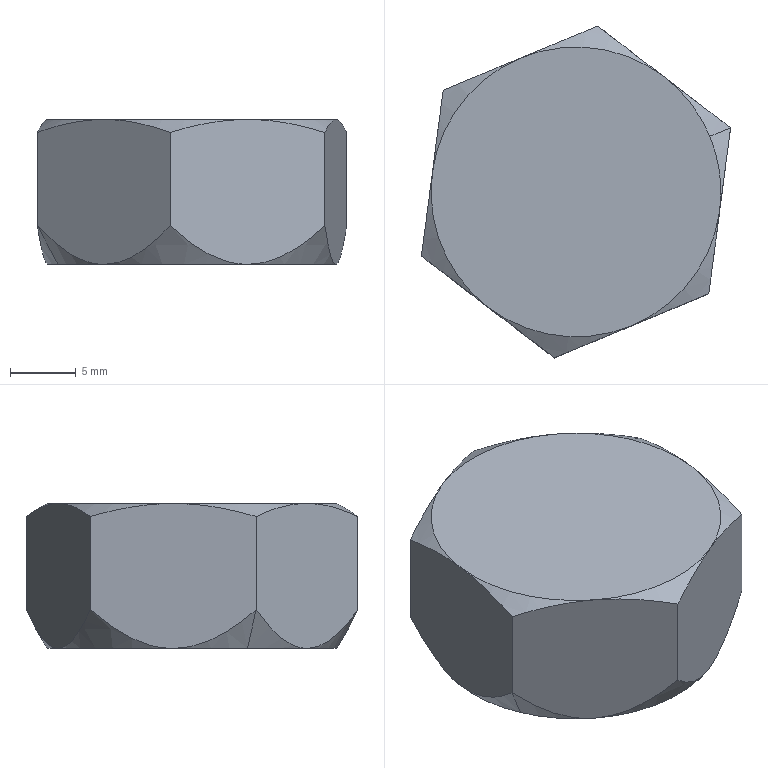Part | SolidWorks | features BaseBody 1 | 1 solid | 30 faces | box 23.463 x 25.189 x 11 mm | volume 2187 mm3 | cone 16 | plane 10 | cylinder 4 | commonest cylinder face diameters 18 x2 19 x2
STEP:
#1=CARTESIAN_POINT('',(-48.302,46.11,95.75));
#2=VERTEX_POINT('',#1);
#3=CARTESIAN_POINT('',(-51.768,50.624,95.75));
#4=VERTEX_POINT('',#3);
#5=CARTESIAN_POINT('',(-58.463,41.896,95.75));
#6=DIRECTION('',(0.,0.,1.));
#7=DIRECTION('',(0.9237,0.383,0.));
#8=AXIS2_PLACEMENT_3D('',#5,#6,#7);
#9=CIRCLE('',#8,11.);
#10=EDGE_CURVE('',#2,#4,#9,.T.);
#11=ORIENTED_EDGE('',*,*,#10,.F.);
#12=CARTESIAN_POINT('',(-46.732,46.761,94.769));
#13=VERTEX_POINT('',#12);
#14=CARTESIAN_POINT('',(-48.302,46.11,95.75));
#15=DIRECTION('',(0.8,0.3317,-0.5));
#16=VECTOR('',#15,1000.);
#17=LINE('',#14,#16);
#18=EDGE_CURVE('',#2,#13,#17,.T.);
#19=ORIENTED_EDGE('',*,*,#18,.T.);
#20=CARTESIAN_POINT('',(-51.768,50.624,95.75));
#21=CARTESIAN_POINT('',(-50.908,49.965,95.75));
#22=CARTESIAN_POINT('',(-50.06,49.314,95.656));
#23=CARTESIAN_POINT('',(-48.383,48.028,95.314));
#24=CARTESIAN_POINT('',(-47.554,47.392,95.068));
#25=CARTESIAN_POINT('',(-46.732,46.761,94.769));
#26=B_SPLINE_CURVE_WITH_KNOTS('',3,(#20,#21,#22,#23,#24,#25),.UNSPECIFIED.,.F.,.F.,(4,2,4),(0.,0.003211,0.006423),.UNSPECIFIED.);
#27=EDGE_CURVE('',#4,#13,#26,.T.);
#28=ORIENTED_EDGE('',*,*,#27,.F.);
#29=EDGE_LOOP('',(#11,#19,#28));
#30=FACE_OUTER_BOUND('',#29,.T.);
#31=CARTESIAN_POINT('',(-58.463,41.896,95.75));
#32=DIRECTION('',(0.,0.,-1.));
#33=DIRECTION('',(0.9237,0.383,0.));
#34=AXIS2_PLACEMENT_3D('',#31,#32,#33);
#35=CONICAL_SURFACE('',#34,11.,1.047);
#36=ADVANCED_FACE('',(#30),#35,.T.);
#37=CARTESIAN_POINT('',(-68.624,37.683,84.75));
#38=VERTEX_POINT('',#37);
#39=CARTESIAN_POINT('',(-69.37,43.325,84.75));
#40=VERTEX_POINT('',#39);
#41=CARTESIAN_POINT('',(-58.463,41.896,84.75));
#42=DIRECTION('',(0.,0.,-1.));
#43=DIRECTION('',(-0.9237,-0.383,0.));
#44=AXIS2_PLACEMENT_3D('',#41,#42,#43);
#45=CIRCLE('',#44,11.);
#46=EDGE_CURVE('',#38,#40,#45,.T.);
#47=ORIENTED_EDGE('',*,*,#46,.F.);
#48=CARTESIAN_POINT('',(-70.194,37.031,87.694));
#49=VERTEX_POINT('',#48);
#50=CARTESIAN_POINT('',(-68.624,37.683,84.75));
#51=DIRECTION('',(-0.4619,-0.1915,0.866));
#52=VECTOR('',#51,1000.);
#53=LINE('',#50,#52);
#54=EDGE_CURVE('',#38,#49,#53,.T.);
#55=ORIENTED_EDGE('',*,*,#54,.T.);
#56=CARTESIAN_POINT('',(-69.37,43.325,84.75));
#57=CARTESIAN_POINT('',(-69.448,42.726,84.75));
#58=CARTESIAN_POINT('',(-69.524,42.145,84.836));
#59=CARTESIAN_POINT('',(-69.636,41.292,85.072));
#60=CARTESIAN_POINT('',(-69.673,41.011,85.168));
#61=CARTESIAN_POINT('',(-69.745,40.458,85.392));
#62=CARTESIAN_POINT('',(-69.78,40.19,85.517));
#63=CARTESIAN_POINT('',(-69.883,39.404,85.925));
#64=CARTESIAN_POINT('',(-69.949,38.906,86.24));
#65=CARTESIAN_POINT('',(-70.075,37.944,86.929));
#66=CARTESIAN_POINT('',(-70.135,37.48,87.303));
#67=CARTESIAN_POINT('',(-70.194,37.031,87.694));
#68=B_SPLINE_CURVE_WITH_KNOTS('',3,(#56,#57,#58,#59,#60,#61,#62,#63,#64,#65,#66,#67),.UNSPECIFIED.,.F.,.F.,(4,2,2,2,2,4),(0.,0.001777,0.002666,0.003555,0.005332,0.00711),.UNSPECIFIED.);
#69=EDGE_CURVE('',#40,#49,#68,.T.);
#70=ORIENTED_EDGE('',*,*,#69,.F.);
#71=EDGE_LOOP('',(#47,#55,#70));
#72=FACE_OUTER_BOUND('',#71,.T.);
#73=CARTESIAN_POINT('',(-58.463,41.896,84.75));
#74=DIRECTION('',(0.,0.,1.));
#75=DIRECTION('',(-0.9237,-0.383,0.));
#76=AXIS2_PLACEMENT_3D('',#73,#74,#75);
#77=CONICAL_SURFACE('',#76,11.,0.5236);
#78=ADVANCED_FACE('',(#72),#77,.T.);
#79=CARTESIAN_POINT('',(-66.776,38.449,91.75));
#80=VERTEX_POINT('',#79);
#81=CARTESIAN_POINT('',(-50.149,45.344,91.75));
#82=VERTEX_POINT('',#81);
#83=CARTESIAN_POINT('',(-58.463,41.896,91.75));
#84=DIRECTION('',(0.,0.,1.));
#85=DIRECTION('',(0.9237,0.383,0.));
#86=AXIS2_PLACEMENT_3D('',#83,#84,#85);
#87=CIRCLE('',#86,9.);
#88=EDGE_CURVE('',#80,#82,#87,.T.);
#89=ORIENTED_EDGE('',*,*,#88,.T.);
#90=CARTESIAN_POINT('',(-50.149,45.344,85.75));
#91=VERTEX_POINT('',#90);
#92=CARTESIAN_POINT('',(-50.149,45.344,93.75));
#93=DIRECTION('',(0.,0.,-1.));
#94=VECTOR('',#93,1000.);
#95=LINE('',#92,#94);
#96=EDGE_CURVE('',#82,#91,#95,.T.);
#97=ORIENTED_EDGE('',*,*,#96,.T.);
#98=CARTESIAN_POINT('',(-66.776,38.449,85.75));
#99=VERTEX_POINT('',#98);
#100=CARTESIAN_POINT('',(-58.463,41.896,85.75));
#101=DIRECTION('',(0.,0.,-1.));
#102=DIRECTION('',(0.9237,0.383,0.));
#103=AXIS2_PLACEMENT_3D('',#100,#101,#102);
#104=CIRCLE('',#103,9.);
#105=EDGE_CURVE('',#91,#99,#104,.T.);
#106=ORIENTED_EDGE('',*,*,#105,.T.);
#107=CARTESIAN_POINT('',(-66.776,38.449,93.75));
#108=DIRECTION('',(0.,0.,-1.));
#109=VECTOR('',#108,1000.);
#110=LINE('',#107,#109);
#111=EDGE_CURVE('',#80,#99,#110,.T.);
#112=ORIENTED_EDGE('',*,*,#111,.F.);
#113=EDGE_LOOP('',(#89,#97,#106,#112));
#114=FACE_OUTER_BOUND('',#113,.T.);
#115=CARTESIAN_POINT('',(-58.463,41.896,93.75));
#116=DIRECTION('',(0.,0.,-1.));
#117=DIRECTION('',(-0.9237,-0.383,0.));
#118=AXIS2_PLACEMENT_3D('',#115,#116,#117);
#119=CYLINDRICAL_SURFACE('',#118,9.);
#120=ADVANCED_FACE('',(#114),#119,.F.);
#121=CARTESIAN_POINT('',(-67.238,38.257,91.75));
#122=VERTEX_POINT('',#121);
#123=CARTESIAN_POINT('',(-49.687,45.535,91.75));
#124=VERTEX_POINT('',#123);
#125=CARTESIAN_POINT('',(-58.463,41.896,91.75));
#126=DIRECTION('',(0.,0.,1.));
#127=DIRECTION('',(0.9237,0.383,0.));
#128=AXIS2_PLACEMENT_3D('',#125,#126,#127);
#129=CIRCLE('',#128,9.5);
#130=EDGE_CURVE('',#122,#124,#129,.T.);
#131=ORIENTED_EDGE('',*,*,#130,.F.);
#132=CARTESIAN_POINT('',(-67.238,38.257,93.75));
#133=VERTEX_POINT('',#132);
#134=CARTESIAN_POINT('',(-67.238,38.257,91.75));
#135=DIRECTION('',(0.,0.,1.));
#136=VECTOR('',#135,1000.);
#137=LINE('',#134,#136);
#138=EDGE_CURVE('',#122,#133,#137,.T.);
#139=ORIENTED_EDGE('',*,*,#138,.T.);
#140=CARTESIAN_POINT('',(-49.687,45.535,93.75));
#141=VERTEX_POINT('',#140);
#142=CARTESIAN_POINT('',(-58.463,41.896,93.75));
#143=DIRECTION('',(0.,0.,1.));
#144=DIRECTION('',(0.9237,0.383,0.));
#145=AXIS2_PLACEMENT_3D('',#142,#143,#144);
#146=CIRCLE('',#145,9.5);
#147=EDGE_CURVE('',#133,#141,#146,.T.);
#148=ORIENTED_EDGE('',*,*,#147,.T.);
#149=CARTESIAN_POINT('',(-49.687,45.535,91.75));
#150=DIRECTION('',(0.,0.,1.));
#151=VECTOR('',#150,1000.);
#152=LINE('',#149,#151);
#153=EDGE_CURVE('',#124,#141,#152,.T.);
#154=ORIENTED_EDGE('',*,*,#153,.F.);
#155=EDGE_LOOP('',(#131,#139,#148,#154));
#156=FACE_OUTER_BOUND('',#155,.T.);
#157=CARTESIAN_POINT('',(-58.463,41.896,91.75));
#158=DIRECTION('',(0.,0.,1.));
#159=DIRECTION('',(0.9237,0.383,0.));
#160=AXIS2_PLACEMENT_3D('',#157,#158,#159);
#161=CYLINDRICAL_SURFACE('',#160,9.5);
#162=ADVANCED_FACE('',(#156),#161,.F.);
#163=ORIENTED_EDGE('',*,*,#105,.F.);
#164=CARTESIAN_POINT('',(-49.226,45.727,84.75));
#165=VERTEX_POINT('',#164);
#166=CARTESIAN_POINT('',(-50.149,45.344,85.75));
#167=DIRECTION('',(0.6532,0.2709,-0.7071));
#168=VECTOR('',#167,1000.);
#169=LINE('',#166,#168);
#170=EDGE_CURVE('',#91,#165,#169,.T.);
#171=ORIENTED_EDGE('',*,*,#170,.T.);
#172=CARTESIAN_POINT('',(-67.7,38.066,84.75));
#173=VERTEX_POINT('',#172);
#174=CARTESIAN_POINT('',(-58.463,41.896,84.75));
#175=DIRECTION('',(0.,0.,1.));
#176=DIRECTION('',(0.9237,0.383,0.));
#177=AXIS2_PLACEMENT_3D('',#174,#175,#176);
#178=CIRCLE('',#177,10.);
#179=EDGE_CURVE('',#173,#165,#178,.T.);
#180=ORIENTED_EDGE('',*,*,#179,.F.);
#181=CARTESIAN_POINT('',(-66.776,38.449,85.75));
#182=DIRECTION('',(-0.6532,-0.2709,-0.7071));
#183=VECTOR('',#182,1000.);
#184=LINE('',#181,#183);
#185=EDGE_CURVE('',#99,#173,#184,.T.);
#186=ORIENTED_EDGE('',*,*,#185,.F.);
#187=EDGE_LOOP('',(#163,#171,#180,#186));
#188=FACE_OUTER_BOUND('',#187,.T.);
#189=CARTESIAN_POINT('',(-58.463,41.896,85.75));
#190=DIRECTION('',(0.,0.,-1.));
#191=DIRECTION('',(-0.9237,-0.383,0.));
#192=AXIS2_PLACEMENT_3D('',#189,#190,#191);
#193=CONICAL_SURFACE('',#192,9.,0.7854);
#194=ADVANCED_FACE('',(#188),#193,.F.);
#195=ORIENTED_EDGE('',*,*,#170,.F.);
#196=CARTESIAN_POINT('',(-58.463,41.896,85.75));
#197=DIRECTION('',(0.,0.,-1.));
#198=DIRECTION('',(0.9237,0.383,0.));
#199=AXIS2_PLACEMENT_3D('',#196,#197,#198);
#200=CIRCLE('',#199,9.);
#201=EDGE_CURVE('',#99,#91,#200,.T.);
#202=ORIENTED_EDGE('',*,*,#201,.F.);
#203=ORIENTED_EDGE('',*,*,#185,.T.);
#204=CARTESIAN_POINT('',(-58.463,41.896,84.75));
#205=DIRECTION('',(0.,0.,1.));
#206=DIRECTION('',(0.9237,0.383,0.));
#207=AXIS2_PLACEMENT_3D('',#204,#205,#206);
#208=CIRCLE('',#207,10.);
#209=EDGE_CURVE('',#165,#173,#208,.T.);
#210=ORIENTED_EDGE('',*,*,#209,.F.);
#211=EDGE_LOOP('',(#195,#202,#203,#210));
#212=FACE_OUTER_BOUND('',#211,.T.);
#213=CARTESIAN_POINT('',(-58.463,41.896,85.75));
#214=DIRECTION('',(0.,0.,-1.));
#215=DIRECTION('',(-0.9237,-0.383,0.));
#216=AXIS2_PLACEMENT_3D('',#213,#214,#215);
#217=CONICAL_SURFACE('',#216,9.,0.7854);
#218=ADVANCED_FACE('',(#212),#217,.F.);
#219=CARTESIAN_POINT('',(-58.463,41.896,93.75));
#220=DIRECTION('',(0.,0.,1.));
#221=DIRECTION('',(0.9237,0.383,0.));
#222=AXIS2_PLACEMENT_3D('',#219,#220,#221);
#223=CIRCLE('',#222,9.5);
#224=EDGE_CURVE('',#141,#133,#223,.T.);
#225=ORIENTED_EDGE('',*,*,#224,.F.);
#226=ORIENTED_EDGE('',*,*,#147,.F.);
#227=EDGE_LOOP('',(#225,#226));
#228=FACE_OUTER_BOUND('',#227,.T.);
#229=CARTESIAN_POINT('',(-58.463,41.896,93.75));
#230=DIRECTION('',(0.,0.,1.));
#231=DIRECTION('',(1.,0.,0.));
#232=AXIS2_PLACEMENT_3D('',#229,#230,#231);
#233=PLANE('',#232);
#234=ADVANCED_FACE('',(#228),#233,.F.);
#235=CARTESIAN_POINT('',(-58.463,41.896,91.75));
#236=DIRECTION('',(0.,0.,1.));
#237=DIRECTION('',(0.9237,0.383,0.));
#238=AXIS2_PLACEMENT_3D('',#235,#236,#237);
#239=CIRCLE('',#238,9.5);
#240=EDGE_CURVE('',#124,#122,#239,.T.);
#241=ORIENTED_EDGE('',*,*,#240,.T.);
#242=ORIENTED_EDGE('',*,*,#130,.T.);
#243=EDGE_LOOP('',(#241,#242));
#244=FACE_OUTER_BOUND('',#243,.T.);
#245=ORIENTED_EDGE('',*,*,#88,.F.);
#246=CARTESIAN_POINT('',(-58.463,41.896,91.75));
#247=DIRECTION('',(0.,0.,1.));
#248=DIRECTION('',(0.9237,0.383,0.));
#249=AXIS2_PLACEMENT_3D('',#246,#247,#248);
#250=CIRCLE('',#249,9.);
#251=EDGE_CURVE('',#82,#80,#250,.T.);
#252=ORIENTED_EDGE('',*,*,#251,.F.);
#253=EDGE_LOOP('',(#245,#252));
#254=FACE_BOUND('',#253,.T.);
#255=CARTESIAN_POINT('',(-58.463,41.896,91.75));
#256=DIRECTION('',(0.,0.,1.));
#257=DIRECTION('',(1.,0.,0.));
#258=AXIS2_PLACEMENT_3D('',#255,#256,#257);
#259=PLANE('',#258);
#260=ADVANCED_FACE('',(#244,#254),#259,.T.);
#261=ORIENTED_EDGE('',*,*,#138,.F.);
#262=ORIENTED_EDGE('',*,*,#240,.F.);
#263=ORIENTED_EDGE('',*,*,#153,.T.);
#264=ORIENTED_EDGE('',*,*,#224,.T.);
#265=EDGE_LOOP('',(#261,#262,#263,#264));
#266=FACE_OUTER_BOUND('',#265,.T.);
#267=CARTESIAN_POINT('',(-58.463,41.896,91.75));
#268=DIRECTION('',(0.,0.,1.));
#269=DIRECTION('',(0.9237,0.383,0.));
#270=AXIS2_PLACEMENT_3D('',#267,#268,#269);
#271=CYLINDRICAL_SURFACE('',#270,9.5);
#272=ADVANCED_FACE('',(#266),#271,.F.);
#273=ORIENTED_EDGE('',*,*,#96,.F.);
#274=ORIENTED_EDGE('',*,*,#251,.T.);
#275=ORIENTED_EDGE('',*,*,#111,.T.);
#276=ORIENTED_EDGE('',*,*,#201,.T.);
#277=EDGE_LOOP('',(#273,#274,#275,#276));
#278=FACE_OUTER_BOUND('',#277,.T.);
#279=CARTESIAN_POINT('',(-58.463,41.896,93.75));
#280=DIRECTION('',(0.,0.,-1.));
#281=DIRECTION('',(-0.9237,-0.383,0.));
#282=AXIS2_PLACEMENT_3D('',#279,#280,#281);
#283=CYLINDRICAL_SURFACE('',#282,9.);
#284=ADVANCED_FACE('',(#278),#283,.F.);
#285=CARTESIAN_POINT('',(-56.808,54.491,87.699));
#286=VERTEX_POINT('',#285);
#287=CARTESIAN_POINT('',(-62.676,52.057,84.75));
#288=VERTEX_POINT('',#287);
#289=CARTESIAN_POINT('',(-56.808,54.491,87.699));
#290=CARTESIAN_POINT('',(-57.226,54.318,87.308));
#291=CARTESIAN_POINT('',(-57.655,54.14,86.936));
#292=CARTESIAN_POINT('',(-58.548,53.769,86.249));
#293=CARTESIAN_POINT('',(-59.011,53.577,85.933));
#294=CARTESIAN_POINT('',(-59.744,53.273,85.523));
#295=CARTESIAN_POINT('',(-59.996,53.169,85.396));
#296=CARTESIAN_POINT('',(-60.511,52.955,85.172));
#297=CARTESIAN_POINT('',(-60.772,52.847,85.076));
#298=CARTESIAN_POINT('',(-61.302,52.627,84.917));
#299=CARTESIAN_POINT('',(-61.571,52.516,84.856));
#300=CARTESIAN_POINT('',(-62.118,52.289,84.772));
#301=CARTESIAN_POINT('',(-62.397,52.173,84.75));
#302=CARTESIAN_POINT('',(-62.676,52.057,84.75));
#303=B_SPLINE_CURVE_WITH_KNOTS('',3,(#289,#290,#291,#292,#293,#294,#295,#296,#297,#298,#299,#300,#301,#302),.UNSPECIFIED.,.F.,.F.,(4,2,2,2,2,2,4),(0.,0.001777,0.003555,0.004444,0.005332,0.006221,0.00711),.UNSPECIFIED.);
#304=EDGE_CURVE('',#286,#288,#303,.T.);
#305=ORIENTED_EDGE('',*,*,#304,.F.);
#306=CARTESIAN_POINT('',(-51.768,50.624,84.75));
#307=VERTEX_POINT('',#306);
#308=CARTESIAN_POINT('',(-51.768,50.624,84.75));
#309=CARTESIAN_POINT('',(-52.247,50.992,84.75));
#310=CARTESIAN_POINT('',(-52.714,51.35,84.836));
#311=CARTESIAN_POINT('',(-53.396,51.873,85.072));
#312=CARTESIAN_POINT('',(-53.622,52.046,85.169));
#313=CARTESIAN_POINT('',(-54.064,52.386,85.393));
#314=CARTESIAN_POINT('',(-54.279,52.551,85.518));
#315=CARTESIAN_POINT('',(-54.909,53.033,85.927));
#316=CARTESIAN_POINT('',(-55.307,53.339,86.243));
#317=CARTESIAN_POINT('',(-56.078,53.93,86.932));
#318=CARTESIAN_POINT('',(-56.449,54.215,87.307));
#319=CARTESIAN_POINT('',(-56.808,54.491,87.699));
#320=B_SPLINE_CURVE_WITH_KNOTS('',3,(#308,#309,#310,#311,#312,#313,#314,#315,#316,#317,#318,#319),.UNSPECIFIED.,.F.,.F.,(4,2,2,2,2,4),(0.,0.001779,0.002669,0.003558,0.005337,0.007116),.UNSPECIFIED.);
#321=EDGE_CURVE('',#307,#286,#320,.T.);
#322=ORIENTED_EDGE('',*,*,#321,.F.);
#323=CARTESIAN_POINT('',(-58.463,41.896,84.75));
#324=DIRECTION('',(0.,0.,-1.));
#325=DIRECTION('',(-0.9237,-0.383,0.));
#326=AXIS2_PLACEMENT_3D('',#323,#324,#325);
#327=CIRCLE('',#326,11.);
#328=EDGE_CURVE('',#288,#307,#327,.T.);
#329=ORIENTED_EDGE('',*,*,#328,.F.);
#330=EDGE_LOOP('',(#305,#322,#329));
#331=FACE_OUTER_BOUND('',#330,.T.);
#332=CARTESIAN_POINT('',(-58.463,41.896,84.75));
#333=DIRECTION('',(0.,0.,1.));
#334=DIRECTION('',(-0.9237,-0.383,0.));
#335=AXIS2_PLACEMENT_3D('',#332,#333,#334);
#336=CONICAL_SURFACE('',#335,11.,0.5236);
#337=ADVANCED_FACE('',(#331),#336,.T.);
#338=CARTESIAN_POINT('',(-68.544,49.624,87.699));
#339=VERTEX_POINT('',#338);
#340=CARTESIAN_POINT('',(-62.676,52.057,84.75));
#341=CARTESIAN_POINT('',(-63.235,51.826,84.75));
#342=CARTESIAN_POINT('',(-63.777,51.601,84.836));
#343=CARTESIAN_POINT('',(-64.572,51.271,85.072));
#344=CARTESIAN_POINT('',(-64.834,51.162,85.169));
#345=CARTESIAN_POINT('',(-65.35,50.949,85.393));
#346=CARTESIAN_POINT('',(-65.6,50.845,85.518));
#347=CARTESIAN_POINT('',(-66.333,50.541,85.927));
#348=CARTESIAN_POINT('',(-66.797,50.348,86.243));
#349=CARTESIAN_POINT('',(-67.694,49.977,86.932));
#350=CARTESIAN_POINT('',(-68.126,49.797,87.307));
#351=CARTESIAN_POINT('',(-68.544,49.624,87.699));
#352=B_SPLINE_CURVE_WITH_KNOTS('',3,(#340,#341,#342,#343,#344,#345,#346,#347,#348,#349,#350,#351),.UNSPECIFIED.,.F.,.F.,(4,2,2,2,2,4),(0.,0.001779,0.002669,0.003558,0.005337,0.007116),.UNSPECIFIED.);
#353=EDGE_CURVE('',#288,#339,#352,.T.);
#354=ORIENTED_EDGE('',*,*,#353,.F.);
#355=CARTESIAN_POINT('',(-58.463,41.896,84.75));
#356=DIRECTION('',(0.,0.,-1.));
#357=DIRECTION('',(-0.9237,-0.383,0.));
#358=AXIS2_PLACEMENT_3D('',#355,#356,#357);
#359=CIRCLE('',#358,11.);
#360=EDGE_CURVE('',#40,#288,#359,.T.);
#361=ORIENTED_EDGE('',*,*,#360,.F.);
#362=CARTESIAN_POINT('',(-68.544,49.624,87.699));
#363=CARTESIAN_POINT('',(-68.603,49.176,87.308));
#364=CARTESIAN_POINT('',(-68.663,48.715,86.936));
#365=CARTESIAN_POINT('',(-68.789,47.757,86.249));
#366=CARTESIAN_POINT('',(-68.854,47.26,85.933));
#367=CARTESIAN_POINT('',(-68.957,46.473,85.523));
#368=CARTESIAN_POINT('',(-68.993,46.202,85.396));
#369=CARTESIAN_POINT('',(-69.065,45.649,85.172));
#370=CARTESIAN_POINT('',(-69.102,45.369,85.076));
#371=CARTESIAN_POINT('',(-69.176,44.801,84.917));
#372=CARTESIAN_POINT('',(-69.214,44.512,84.856));
#373=CARTESIAN_POINT('',(-69.291,43.924,84.772));
#374=CARTESIAN_POINT('',(-69.33,43.625,84.75));
#375=CARTESIAN_POINT('',(-69.37,43.325,84.75));
#376=B_SPLINE_CURVE_WITH_KNOTS('',3,(#362,#363,#364,#365,#366,#367,#368,#369,#370,#371,#372,#373,#374,#375),.UNSPECIFIED.,.F.,.F.,(4,2,2,2,2,2,4),(0.,0.001777,0.003555,0.004444,0.005332,0.006221,0.00711),.UNSPECIFIED.);
#377=EDGE_CURVE('',#339,#40,#376,.T.);
#378=ORIENTED_EDGE('',*,*,#377,.F.);
#379=EDGE_LOOP('',(#354,#361,#378));
#380=FACE_OUTER_BOUND('',#379,.T.);
#381=CARTESIAN_POINT('',(-58.463,41.896,84.75));
#382=DIRECTION('',(0.,0.,1.));
#383=DIRECTION('',(-0.9237,-0.383,0.));
#384=AXIS2_PLACEMENT_3D('',#381,#382,#383);
#385=CONICAL_SURFACE('',#384,11.,0.5236);
#386=ADVANCED_FACE('',(#380),#385,.T.);
#387=ORIENTED_EDGE('',*,*,#54,.F.);
#388=CARTESIAN_POINT('',(-65.158,33.168,84.75));
#389=VERTEX_POINT('',#388);
#390=CARTESIAN_POINT('',(-58.463,41.896,84.75));
#391=DIRECTION('',(0.,0.,-1.));
#392=DIRECTION('',(-0.9237,-0.383,0.));
#393=AXIS2_PLACEMENT_3D('',#390,#391,#392);
#394=CIRCLE('',#393,11.);
#395=EDGE_CURVE('',#389,#38,#394,.T.);
#396=ORIENTED_EDGE('',*,*,#395,.F.);
#397=CARTESIAN_POINT('',(-70.194,37.031,87.694));
#398=CARTESIAN_POINT('',(-69.836,36.757,87.304));
#399=CARTESIAN_POINT('',(-69.468,36.474,86.932));
#400=CARTESIAN_POINT('',(-68.701,35.886,86.246));
#401=CARTESIAN_POINT('',(-68.304,35.581,85.931));
#402=CARTESIAN_POINT('',(-67.674,35.099,85.521));
#403=CARTESIAN_POINT('',(-67.458,34.933,85.395));
#404=CARTESIAN_POINT('',(-67.016,34.594,85.171));
#405=CARTESIAN_POINT('',(-66.792,34.422,85.075));
#406=CARTESIAN_POINT('',(-66.337,34.073,84.917));
#407=CARTESIAN_POINT('',(-66.107,33.896,84.855));
#408=CARTESIAN_POINT('',(-65.637,33.536,84.772));
#409=CARTESIAN_POINT('',(-65.397,33.352,84.75));
#410=CARTESIAN_POINT('',(-65.158,33.168,84.75));
#411=B_SPLINE_CURVE_WITH_KNOTS('',3,(#397,#398,#399,#400,#401,#402,#403,#404,#405,#406,#407,#408,#409,#410),.UNSPECIFIED.,.F.,.F.,(4,2,2,2,2,2,4),(0.,0.001776,0.003552,0.004439,0.005327,0.006215,0.007103),.UNSPECIFIED.);
#412=EDGE_CURVE('',#49,#389,#411,.T.);
#413=ORIENTED_EDGE('',*,*,#412,.F.);
#414=EDGE_LOOP('',(#387,#396,#413));
#415=FACE_OUTER_BOUND('',#414,.T.);
#416=CARTESIAN_POINT('',(-58.463,41.896,84.75));
#417=DIRECTION('',(0.,0.,1.));
#418=DIRECTION('',(-0.9237,-0.383,0.));
#419=AXIS2_PLACEMENT_3D('',#416,#417,#418);
#420=CONICAL_SURFACE('',#419,11.,0.5236);
#421=ADVANCED_FACE('',(#415),#420,.T.);
#422=CARTESIAN_POINT('',(-46.732,46.761,87.694));
#423=VERTEX_POINT('',#422);
#424=CARTESIAN_POINT('',(-46.732,46.761,87.694));
#425=CARTESIAN_POINT('',(-47.09,47.036,87.304));
#426=CARTESIAN_POINT('',(-47.458,47.318,86.932));
#427=CARTESIAN_POINT('',(-48.224,47.906,86.246));
#428=CARTESIAN_POINT('',(-48.622,48.211,85.931));
#429=CARTESIAN_POINT('',(-49.251,48.694,85.521));
#430=CARTESIAN_POINT('',(-49.468,48.86,85.395));
#431=CARTESIAN_POINT('',(-49.91,49.199,85.171));
#432=CARTESIAN_POINT('',(-50.134,49.371,85.075));
#433=CARTESIAN_POINT('',(-50.588,49.719,84.917));
#434=CARTESIAN_POINT('',(-50.819,49.896,84.855));
#435=CARTESIAN_POINT('',(-51.289,50.257,84.772));
#436=CARTESIAN_POINT('',(-51.528,50.441,84.75));
#437=CARTESIAN_POINT('',(-51.768,50.624,84.75));
#438=B_SPLINE_CURVE_WITH_KNOTS('',3,(#424,#425,#426,#427,#428,#429,#430,#431,#432,#433,#434,#435,#436,#437),.UNSPECIFIED.,.F.,.F.,(4,2,2,2,2,2,4),(0.,0.001776,0.003552,0.004439,0.005327,0.006215,0.007103),.UNSPECIFIED.);
#439=EDGE_CURVE('',#423,#307,#438,.T.);
#440=ORIENTED_EDGE('',*,*,#439,.F.);
#441=CARTESIAN_POINT('',(-47.556,40.467,84.75));
#442=VERTEX_POINT('',#441);
#443=CARTESIAN_POINT('',(-47.556,40.467,84.75));
#444=CARTESIAN_POINT('',(-47.478,41.066,84.75));
#445=CARTESIAN_POINT('',(-47.401,41.648,84.836));
#446=CARTESIAN_POINT('',(-47.29,42.5,85.072));
#447=CARTESIAN_POINT('',(-47.253,42.781,85.168));
#448=CARTESIAN_POINT('',(-47.18,43.334,85.392));
#449=CARTESIAN_POINT('',(-47.145,43.603,85.517));
#450=CARTESIAN_POINT('',(-47.042,44.389,85.925));
#451=CARTESIAN_POINT('',(-46.977,44.887,86.24));
#452=CARTESIAN_POINT('',(-46.851,45.848,86.929));
#453=CARTESIAN_POINT('',(-46.79,46.313,87.303));
#454=CARTESIAN_POINT('',(-46.732,46.761,87.694));
#455=B_SPLINE_CURVE_WITH_KNOTS('',3,(#443,#444,#445,#446,#447,#448,#449,#450,#451,#452,#453,#454),.UNSPECIFIED.,.F.,.F.,(4,2,2,2,2,4),(0.,0.001777,0.002666,0.003555,0.005332,0.00711),.UNSPECIFIED.);
#456=EDGE_CURVE('',#442,#423,#455,.T.);
#457=ORIENTED_EDGE('',*,*,#456,.F.);
#458=CARTESIAN_POINT('',(-58.463,41.896,84.75));
#459=DIRECTION('',(0.,0.,-1.));
#460=DIRECTION('',(-0.9237,-0.383,0.));
#461=AXIS2_PLACEMENT_3D('',#458,#459,#460);
#462=CIRCLE('',#461,11.);
#463=EDGE_CURVE('',#307,#442,#462,.T.);
#464=ORIENTED_EDGE('',*,*,#463,.F.);
#465=EDGE_LOOP('',(#440,#457,#464));
#466=FACE_OUTER_BOUND('',#465,.T.);
#467=CARTESIAN_POINT('',(-58.463,41.896,84.75));
#468=DIRECTION('',(0.,0.,1.));
#469=DIRECTION('',(-0.9237,-0.383,0.));
#470=AXIS2_PLACEMENT_3D('',#467,#468,#469);
#471=CONICAL_SURFACE('',#470,11.,0.5236);
#472=ADVANCED_FACE('',(#466),#471,.T.);
#473=CARTESIAN_POINT('',(-60.117,29.302,87.699));
#474=VERTEX_POINT('',#473);
#475=CARTESIAN_POINT('',(-65.158,33.168,84.75));
#476=CARTESIAN_POINT('',(-64.678,32.8,84.75));
#477=CARTESIAN_POINT('',(-64.212,32.443,84.836));
#478=CARTESIAN_POINT('',(-63.53,31.919,85.072));
#479=CARTESIAN_POINT('',(-63.304,31.746,85.169));
#480=CARTESIAN_POINT('',(-62.861,31.407,85.393));
#481=CARTESIAN_POINT('',(-62.646,31.242,85.518));
#482=CARTESIAN_POINT('',(-62.017,30.759,85.927));
#483=CARTESIAN_POINT('',(-61.618,30.453,86.243));
#484=CARTESIAN_POINT('',(-60.848,29.862,86.932));
#485=CARTESIAN_POINT('',(-60.476,29.577,87.307));
#486=CARTESIAN_POINT('',(-60.117,29.302,87.699));
#487=B_SPLINE_CURVE_WITH_KNOTS('',3,(#475,#476,#477,#478,#479,#480,#481,#482,#483,#484,#485,#486),.UNSPECIFIED.,.F.,.F.,(4,2,2,2,2,4),(0.,0.001779,0.002669,0.003558,0.005337,0.007116),.UNSPECIFIED.);
#488=EDGE_CURVE('',#389,#474,#487,.T.);
#489=ORIENTED_EDGE('',*,*,#488,.F.);
#490=CARTESIAN_POINT('',(-54.249,31.735,84.75));
#491=VERTEX_POINT('',#490);
#492=CARTESIAN_POINT('',(-58.463,41.896,84.75));
#493=DIRECTION('',(0.,0.,-1.));
#494=DIRECTION('',(-0.9237,-0.383,0.));
#495=AXIS2_PLACEMENT_3D('',#492,#493,#494);
#496=CIRCLE('',#495,11.);
#497=EDGE_CURVE('',#491,#389,#496,.T.);
#498=ORIENTED_EDGE('',*,*,#497,.F.);
#499=CARTESIAN_POINT('',(-60.117,29.302,87.699));
#500=CARTESIAN_POINT('',(-59.7,29.475,87.308));
#501=CARTESIAN_POINT('',(-59.271,29.653,86.936));
#502=CARTESIAN_POINT('',(-58.378,30.023,86.249));
#503=CARTESIAN_POINT('',(-57.915,30.215,85.933));
#504=CARTESIAN_POINT('',(-57.182,30.519,85.523));
#505=CARTESIAN_POINT('',(-56.929,30.624,85.396));
#506=CARTESIAN_POINT('',(-56.415,30.837,85.172));
#507=CARTESIAN_POINT('',(-56.154,30.945,85.076));
#508=CARTESIAN_POINT('',(-55.624,31.165,84.917));
#509=CARTESIAN_POINT('',(-55.355,31.277,84.856));
#510=CARTESIAN_POINT('',(-54.808,31.504,84.772));
#511=CARTESIAN_POINT('',(-54.528,31.62,84.75));
#512=CARTESIAN_POINT('',(-54.249,31.735,84.75));
#513=B_SPLINE_CURVE_WITH_KNOTS('',3,(#499,#500,#501,#502,#503,#504,#505,#506,#507,#508,#509,#510,#511,#512),.UNSPECIFIED.,.F.,.F.,(4,2,2,2,2,2,4),(0.,0.001777,0.003555,0.004444,0.005332,0.006221,0.00711),.UNSPECIFIED.);
#514=EDGE_CURVE('',#474,#491,#513,.T.);
#515=ORIENTED_EDGE('',*,*,#514,.F.);
#516=EDGE_LOOP('',(#489,#498,#515));
#517=FACE_OUTER_BOUND('',#516,.T.);
#518=CARTESIAN_POINT('',(-58.463,41.896,84.75));
#519=DIRECTION('',(0.,0.,1.));
#520=DIRECTION('',(-0.9237,-0.383,0.));
#521=AXIS2_PLACEMENT_3D('',#518,#519,#520);
#522=CONICAL_SURFACE('',#521,11.,0.5236);
#523=ADVANCED_FACE('',(#517),#522,.T.);
#524=ORIENTED_EDGE('',*,*,#328,.T.);
#525=ORIENTED_EDGE('',*,*,#463,.T.);
#526=CARTESIAN_POINT('',(-58.463,41.896,84.75));
#527=DIRECTION('',(0.,0.,-1.));
#528=DIRECTION('',(-0.9237,-0.383,0.));
#529=AXIS2_PLACEMENT_3D('',#526,#527,#528);
#530=CIRCLE('',#529,11.);
#531=EDGE_CURVE('',#442,#491,#530,.T.);
#532=ORIENTED_EDGE('',*,*,#531,.T.);
#533=ORIENTED_EDGE('',*,*,#497,.T.);
#534=ORIENTED_EDGE('',*,*,#395,.T.);
#535=ORIENTED_EDGE('',*,*,#46,.T.);
#536=ORIENTED_EDGE('',*,*,#360,.T.);
#537=EDGE_LOOP('',(#524,#525,#532,#533,#534,#535,#536));
#538=FACE_OUTER_BOUND('',#537,.T.);
#539=ORIENTED_EDGE('',*,*,#179,.T.);
#540=ORIENTED_EDGE('',*,*,#209,.T.);
#541=EDGE_LOOP('',(#539,#540));
#542=FACE_BOUND('',#541,.T.);
#543=CARTESIAN_POINT('',(-80.271,44.761,84.75));
#544=DIRECTION('',(0.,0.,1.));
#545=DIRECTION('',(1.,0.,0.));
#546=AXIS2_PLACEMENT_3D('',#543,#544,#545);
#547=PLANE('',#546);
#548=ADVANCED_FACE('',(#538,#542),#547,.F.);
#549=CARTESIAN_POINT('',(-48.381,34.169,87.699));
#550=VERTEX_POINT('',#549);
#551=CARTESIAN_POINT('',(-48.381,34.169,87.699));
#552=CARTESIAN_POINT('',(-48.323,34.616,87.308));
#553=CARTESIAN_POINT('',(-48.262,35.077,86.936));
#554=CARTESIAN_POINT('',(-48.137,36.035,86.249));
#555=CARTESIAN_POINT('',(-48.072,36.533,85.933));
#556=CARTESIAN_POINT('',(-47.968,37.32,85.523));
#557=CARTESIAN_POINT('',(-47.933,37.59,85.396));
#558=CARTESIAN_POINT('',(-47.861,38.143,85.172));
#559=CARTESIAN_POINT('',(-47.824,38.423,85.076));
#560=CARTESIAN_POINT('',(-47.749,38.992,84.917));
#561=CARTESIAN_POINT('',(-47.712,39.281,84.856));
#562=CARTESIAN_POINT('',(-47.635,39.868,84.772));
#563=CARTESIAN_POINT('',(-47.595,40.168,84.75));
#564=CARTESIAN_POINT('',(-47.556,40.467,84.75));
#565=B_SPLINE_CURVE_WITH_KNOTS('',3,(#551,#552,#553,#554,#555,#556,#557,#558,#559,#560,#561,#562,#563,#564),.UNSPECIFIED.,.F.,.F.,(4,2,2,2,2,2,4),(0.,0.001777,0.003555,0.004444,0.005332,0.006221,0.00711),.UNSPECIFIED.);
#566=EDGE_CURVE('',#550,#442,#565,.T.);
#567=ORIENTED_EDGE('',*,*,#566,.F.);
#568=CARTESIAN_POINT('',(-54.249,31.735,84.75));
#569=CARTESIAN_POINT('',(-53.691,31.967,84.75));
#570=CARTESIAN_POINT('',(-53.148,32.192,84.836));
#571=CARTESIAN_POINT('',(-52.354,32.521,85.072));
#572=CARTESIAN_POINT('',(-52.091,32.63,85.169));
#573=CARTESIAN_POINT('',(-51.576,32.844,85.393));
#574=CARTESIAN_POINT('',(-51.326,32.948,85.518));
#575=CARTESIAN_POINT('',(-50.593,33.251,85.927));
#576=CARTESIAN_POINT('',(-50.129,33.444,86.243));
#577=CARTESIAN_POINT('',(-49.232,33.816,86.932));
#578=CARTESIAN_POINT('',(-48.799,33.995,87.307));
#579=CARTESIAN_POINT('',(-48.381,34.169,87.699));
#580=B_SPLINE_CURVE_WITH_KNOTS('',3,(#568,#569,#570,#571,#572,#573,#574,#575,#576,#577,#578,#579),.UNSPECIFIED.,.F.,.F.,(4,2,2,2,2,4),(0.,0.001779,0.002669,0.003558,0.005337,0.007116),.UNSPECIFIED.);
#581=EDGE_CURVE('',#491,#550,#580,.T.);
#582=ORIENTED_EDGE('',*,*,#581,.F.);
#583=ORIENTED_EDGE('',*,*,#531,.F.);
#584=EDGE_LOOP('',(#567,#582,#583));
#585=FACE_OUTER_BOUND('',#584,.T.);
#586=CARTESIAN_POINT('',(-58.463,41.896,84.75));
#587=DIRECTION('',(0.,0.,1.));
#588=DIRECTION('',(-0.9237,-0.383,0.));
#589=AXIS2_PLACEMENT_3D('',#586,#587,#588);
#590=CONICAL_SURFACE('',#589,11.,0.5236);
#591=ADVANCED_FACE('',(#585),#590,.T.);
#592=CARTESIAN_POINT('',(-69.37,43.325,95.75));
#593=VERTEX_POINT('',#592);
#594=CARTESIAN_POINT('',(-65.158,33.168,95.75));
#595=VERTEX_POINT('',#594);
#596=CARTESIAN_POINT('',(-58.463,41.896,95.75));
#597=DIRECTION('',(0.,0.,1.));
#598=DIRECTION('',(0.9237,0.383,0.));
#599=AXIS2_PLACEMENT_3D('',#596,#597,#598);
#600=CIRCLE('',#599,11.);
#601=EDGE_CURVE('',#593,#595,#600,.T.);
#602=ORIENTED_EDGE('',*,*,#601,.T.);
#603=CARTESIAN_POINT('',(-54.249,31.735,95.75));
#604=VERTEX_POINT('',#603);
#605=CARTESIAN_POINT('',(-58.463,41.896,95.75));
#606=DIRECTION('',(0.,0.,1.));
#607=DIRECTION('',(0.9237,0.383,0.));
#608=AXIS2_PLACEMENT_3D('',#605,#606,#607);
#609=CIRCLE('',#608,11.);
#610=EDGE_CURVE('',#595,#604,#609,.T.);
#611=ORIENTED_EDGE('',*,*,#610,.T.);
#612=CARTESIAN_POINT('',(-47.556,40.467,95.75));
#613=VERTEX_POINT('',#612);
#614=CARTESIAN_POINT('',(-58.463,41.896,95.75));
#615=DIRECTION('',(0.,0.,1.));
#616=DIRECTION('',(0.9237,0.383,0.));
#617=AXIS2_PLACEMENT_3D('',#614,#615,#616);
#618=CIRCLE('',#617,11.);
#619=EDGE_CURVE('',#604,#613,#618,.T.);
#620=ORIENTED_EDGE('',*,*,#619,.T.);
#621=CARTESIAN_POINT('',(-58.463,41.896,95.75));
#622=DIRECTION('',(0.,0.,1.));
#623=DIRECTION('',(0.9237,0.383,0.));
#624=AXIS2_PLACEMENT_3D('',#621,#622,#623);
#625=CIRCLE('',#624,11.);
#626=EDGE_CURVE('',#613,#2,#625,.T.);
#627=ORIENTED_EDGE('',*,*,#626,.T.);
#628=ORIENTED_EDGE('',*,*,#10,.T.);
#629=CARTESIAN_POINT('',(-62.676,52.057,95.75));
#630=VERTEX_POINT('',#629);
#631=CARTESIAN_POINT('',(-58.463,41.896,95.75));
#632=DIRECTION('',(0.,0.,1.));
#633=DIRECTION('',(0.9237,0.383,0.));
#634=AXIS2_PLACEMENT_3D('',#631,#632,#633);
#635=CIRCLE('',#634,11.);
#636=EDGE_CURVE('',#4,#630,#635,.T.);
#637=ORIENTED_EDGE('',*,*,#636,.T.);
#638=CARTESIAN_POINT('',(-58.463,41.896,95.75));
#639=DIRECTION('',(0.,0.,1.));
#640=DIRECTION('',(0.9237,0.383,0.));
#641=AXIS2_PLACEMENT_3D('',#638,#639,#640);
#642=CIRCLE('',#641,11.);
#643=EDGE_CURVE('',#630,#593,#642,.T.);
#644=ORIENTED_EDGE('',*,*,#643,.T.);
#645=EDGE_LOOP('',(#602,#611,#620,#627,#628,#637,#644));
#646=FACE_OUTER_BOUND('',#645,.T.);
#647=CARTESIAN_POINT('',(-80.271,44.761,95.75));
#648=DIRECTION('',(0.,0.,1.));
#649=DIRECTION('',(1.,0.,0.));
#650=AXIS2_PLACEMENT_3D('',#647,#648,#649);
#651=PLANE('',#650);
#652=ADVANCED_FACE('',(#646),#651,.T.);
#653=CARTESIAN_POINT('',(-60.117,29.302,94.767));
#654=VERTEX_POINT('',#653);
#655=CARTESIAN_POINT('',(-60.117,29.302,94.767));
#656=CARTESIAN_POINT('',(-60.941,29.933,95.067));
#657=CARTESIAN_POINT('',(-61.771,30.57,95.314));
#658=CARTESIAN_POINT('',(-63.449,31.857,95.656));
#659=CARTESIAN_POINT('',(-64.298,32.508,95.75));
#660=CARTESIAN_POINT('',(-65.158,33.168,95.75));
#661=B_SPLINE_CURVE_WITH_KNOTS('',3,(#655,#656,#657,#658,#659,#660),.UNSPECIFIED.,.F.,.F.,(4,2,4),(0.,0.003214,0.006428),.UNSPECIFIED.);
#662=EDGE_CURVE('',#654,#595,#661,.T.);
#663=ORIENTED_EDGE('',*,*,#662,.F.);
#664=CARTESIAN_POINT('',(-54.249,31.735,95.75));
#665=CARTESIAN_POINT('',(-55.251,31.32,95.75));
#666=CARTESIAN_POINT('',(-56.239,30.91,95.656));
#667=CARTESIAN_POINT('',(-58.193,30.1,95.314));
#668=CARTESIAN_POINT('',(-59.159,29.699,95.067));
#669=CARTESIAN_POINT('',(-60.117,29.302,94.767));
#670=B_SPLINE_CURVE_WITH_KNOTS('',3,(#664,#665,#666,#667,#668,#669),.UNSPECIFIED.,.F.,.F.,(4,2,4),(0.,0.003214,0.006428),.UNSPECIFIED.);
#671=EDGE_CURVE('',#604,#654,#670,.T.);
#672=ORIENTED_EDGE('',*,*,#671,.F.);
#673=ORIENTED_EDGE('',*,*,#610,.F.);
#674=EDGE_LOOP('',(#663,#672,#673));
#675=FACE_OUTER_BOUND('',#674,.T.);
#676=CARTESIAN_POINT('',(-58.463,41.896,95.75));
#677=DIRECTION('',(0.,0.,-1.));
#678=DIRECTION('',(0.9237,0.383,0.));
#679=AXIS2_PLACEMENT_3D('',#676,#677,#678);
#680=CONICAL_SURFACE('',#679,11.,1.047);
#681=ADVANCED_FACE('',(#675),#680,.T.);
#682=CARTESIAN_POINT('',(-70.194,37.031,94.769));
#683=VERTEX_POINT('',#682);
#684=CARTESIAN_POINT('',(-65.158,33.168,95.75));
#685=CARTESIAN_POINT('',(-66.017,33.828,95.75));
#686=CARTESIAN_POINT('',(-66.865,34.478,95.656));
#687=CARTESIAN_POINT('',(-68.542,35.764,95.314));
#688=CARTESIAN_POINT('',(-69.371,36.4,95.068));
#689=CARTESIAN_POINT('',(-70.194,37.031,94.769));
#690=B_SPLINE_CURVE_WITH_KNOTS('',3,(#684,#685,#686,#687,#688,#689),.UNSPECIFIED.,.F.,.F.,(4,2,4),(0.,0.003211,0.006423),.UNSPECIFIED.);
#691=EDGE_CURVE('',#595,#683,#690,.T.);
#692=ORIENTED_EDGE('',*,*,#691,.F.);
#693=ORIENTED_EDGE('',*,*,#601,.F.);
#694=CARTESIAN_POINT('',(-70.194,37.031,94.769));
#695=CARTESIAN_POINT('',(-70.06,38.06,95.068));
#696=CARTESIAN_POINT('',(-69.924,39.096,95.314));
#697=CARTESIAN_POINT('',(-69.649,41.191,95.656));
#698=CARTESIAN_POINT('',(-69.51,42.251,95.75));
#699=CARTESIAN_POINT('',(-69.37,43.325,95.75));
#700=B_SPLINE_CURVE_WITH_KNOTS('',3,(#694,#695,#696,#697,#698,#699),.UNSPECIFIED.,.F.,.F.,(4,2,4),(0.,0.003211,0.006423),.UNSPECIFIED.);
#701=EDGE_CURVE('',#683,#593,#700,.T.);
#702=ORIENTED_EDGE('',*,*,#701,.F.);
#703=EDGE_LOOP('',(#692,#693,#702));
#704=FACE_OUTER_BOUND('',#703,.T.);
#705=CARTESIAN_POINT('',(-58.463,41.896,95.75));
#706=DIRECTION('',(0.,0.,-1.));
#707=DIRECTION('',(0.9237,0.383,0.));
#708=AXIS2_PLACEMENT_3D('',#705,#706,#707);
#709=CONICAL_SURFACE('',#708,11.,1.047);
#710=ADVANCED_FACE('',(#704),#709,.T.);
#711=CARTESIAN_POINT('',(-68.544,49.624,94.767));
#712=VERTEX_POINT('',#711);
#713=CARTESIAN_POINT('',(-69.37,43.325,95.75));
#714=CARTESIAN_POINT('',(-69.229,44.4,95.75));
#715=CARTESIAN_POINT('',(-69.09,45.461,95.656));
#716=CARTESIAN_POINT('',(-68.815,47.558,95.314));
#717=CARTESIAN_POINT('',(-68.679,48.595,95.067));
#718=CARTESIAN_POINT('',(-68.544,49.624,94.767));
#719=B_SPLINE_CURVE_WITH_KNOTS('',3,(#713,#714,#715,#716,#717,#718),.UNSPECIFIED.,.F.,.F.,(4,2,4),(0.,0.003214,0.006428),.UNSPECIFIED.);
#720=EDGE_CURVE('',#593,#712,#719,.T.);
#721=ORIENTED_EDGE('',*,*,#720,.F.);
#722=ORIENTED_EDGE('',*,*,#643,.F.);
#723=CARTESIAN_POINT('',(-68.544,49.624,94.767));
#724=CARTESIAN_POINT('',(-67.586,50.021,95.067));
#725=CARTESIAN_POINT('',(-66.62,50.422,95.314));
#726=CARTESIAN_POINT('',(-64.666,51.232,95.656));
#727=CARTESIAN_POINT('',(-63.678,51.642,95.75));
#728=CARTESIAN_POINT('',(-62.676,52.057,95.75));
#729=B_SPLINE_CURVE_WITH_KNOTS('',3,(#723,#724,#725,#726,#727,#728),.UNSPECIFIED.,.F.,.F.,(4,2,4),(0.,0.003214,0.006428),.UNSPECIFIED.);
#730=EDGE_CURVE('',#712,#630,#729,.T.);
#731=ORIENTED_EDGE('',*,*,#730,.F.);
#732=EDGE_LOOP('',(#721,#722,#731));
#733=FACE_OUTER_BOUND('',#732,.T.);
#734=CARTESIAN_POINT('',(-58.463,41.896,95.75));
#735=DIRECTION('',(0.,0.,-1.));
#736=DIRECTION('',(0.9237,0.383,0.));
#737=AXIS2_PLACEMENT_3D('',#734,#735,#736);
#738=CONICAL_SURFACE('',#737,11.,1.047);
#739=ADVANCED_FACE('',(#733),#738,.T.);
#740=CARTESIAN_POINT('',(-56.808,54.491,94.767));
#741=VERTEX_POINT('',#740);
#742=CARTESIAN_POINT('',(-62.676,52.057,95.75));
#743=CARTESIAN_POINT('',(-61.675,52.472,95.75));
#744=CARTESIAN_POINT('',(-60.687,52.882,95.656));
#745=CARTESIAN_POINT('',(-58.733,53.692,95.314));
#746=CARTESIAN_POINT('',(-57.767,54.093,95.067));
#747=CARTESIAN_POINT('',(-56.808,54.491,94.767));
#748=B_SPLINE_CURVE_WITH_KNOTS('',3,(#742,#743,#744,#745,#746,#747),.UNSPECIFIED.,.F.,.F.,(4,2,4),(0.,0.003214,0.006428),.UNSPECIFIED.);
#749=EDGE_CURVE('',#630,#741,#748,.T.);
#750=ORIENTED_EDGE('',*,*,#749,.F.);
#751=ORIENTED_EDGE('',*,*,#636,.F.);
#752=CARTESIAN_POINT('',(-56.808,54.491,94.767));
#753=CARTESIAN_POINT('',(-55.985,53.859,95.067));
#754=CARTESIAN_POINT('',(-55.155,53.222,95.314));
#755=CARTESIAN_POINT('',(-53.477,51.935,95.656));
#756=CARTESIAN_POINT('',(-52.628,51.284,95.75));
#757=CARTESIAN_POINT('',(-51.768,50.624,95.75));
#758=B_SPLINE_CURVE_WITH_KNOTS('',3,(#752,#753,#754,#755,#756,#757),.UNSPECIFIED.,.F.,.F.,(4,2,4),(0.,0.003214,0.006428),.UNSPECIFIED.);
#759=EDGE_CURVE('',#741,#4,#758,.T.);
#760=ORIENTED_EDGE('',*,*,#759,.F.);
#761=EDGE_LOOP('',(#750,#751,#760));
#762=FACE_OUTER_BOUND('',#761,.T.);
#763=CARTESIAN_POINT('',(-58.463,41.896,95.75));
#764=DIRECTION('',(0.,0.,-1.));
#765=DIRECTION('',(0.9237,0.383,0.));
#766=AXIS2_PLACEMENT_3D('',#763,#764,#765);
#767=CONICAL_SURFACE('',#766,11.,1.047);
#768=ADVANCED_FACE('',(#762),#767,.T.);
#769=ORIENTED_EDGE('',*,*,#18,.F.);
#770=ORIENTED_EDGE('',*,*,#626,.F.);
#771=CARTESIAN_POINT('',(-46.732,46.761,94.769));
#772=CARTESIAN_POINT('',(-46.866,45.733,95.068));
#773=CARTESIAN_POINT('',(-47.002,44.697,95.314));
#774=CARTESIAN_POINT('',(-47.277,42.601,95.656));
#775=CARTESIAN_POINT('',(-47.415,41.541,95.75));
#776=CARTESIAN_POINT('',(-47.556,40.467,95.75));
#777=B_SPLINE_CURVE_WITH_KNOTS('',3,(#771,#772,#773,#774,#775,#776),.UNSPECIFIED.,.F.,.F.,(4,2,4),(0.,0.003211,0.006423),.UNSPECIFIED.);
#778=EDGE_CURVE('',#13,#613,#777,.T.);
#779=ORIENTED_EDGE('',*,*,#778,.F.);
#780=EDGE_LOOP('',(#769,#770,#779));
#781=FACE_OUTER_BOUND('',#780,.T.);
#782=CARTESIAN_POINT('',(-58.463,41.896,95.75));
#783=DIRECTION('',(0.,0.,-1.));
#784=DIRECTION('',(0.9237,0.383,0.));
#785=AXIS2_PLACEMENT_3D('',#782,#783,#784);
#786=CONICAL_SURFACE('',#785,11.,1.047);
#787=ADVANCED_FACE('',(#781),#786,.T.);
#788=CARTESIAN_POINT('',(-48.381,34.169,94.767));
#789=VERTEX_POINT('',#788);
#790=CARTESIAN_POINT('',(-47.556,40.467,95.75));
#791=CARTESIAN_POINT('',(-47.697,39.392,95.75));
#792=CARTESIAN_POINT('',(-47.836,38.332,95.656));
#793=CARTESIAN_POINT('',(-48.111,36.235,95.314));
#794=CARTESIAN_POINT('',(-48.246,35.198,95.067));
#795=CARTESIAN_POINT('',(-48.381,34.169,94.767));
#796=B_SPLINE_CURVE_WITH_KNOTS('',3,(#790,#791,#792,#793,#794,#795),.UNSPECIFIED.,.F.,.F.,(4,2,4),(0.,0.003214,0.006428),.UNSPECIFIED.);
#797=EDGE_CURVE('',#613,#789,#796,.T.);
#798=ORIENTED_EDGE('',*,*,#797,.F.);
#799=ORIENTED_EDGE('',*,*,#619,.F.);
#800=CARTESIAN_POINT('',(-48.381,34.169,94.767));
#801=CARTESIAN_POINT('',(-49.34,33.771,95.067));
#802=CARTESIAN_POINT('',(-50.306,33.37,95.314));
#803=CARTESIAN_POINT('',(-52.26,32.56,95.656));
#804=CARTESIAN_POINT('',(-53.248,32.15,95.75));
#805=CARTESIAN_POINT('',(-54.249,31.735,95.75));
#806=B_SPLINE_CURVE_WITH_KNOTS('',3,(#800,#801,#802,#803,#804,#805),.UNSPECIFIED.,.F.,.F.,(4,2,4),(0.,0.003214,0.006428),.UNSPECIFIED.);
#807=EDGE_CURVE('',#789,#604,#806,.T.);
#808=ORIENTED_EDGE('',*,*,#807,.F.);
#809=EDGE_LOOP('',(#798,#799,#808));
#810=FACE_OUTER_BOUND('',#809,.T.);
#811=CARTESIAN_POINT('',(-58.463,41.896,95.75));
#812=DIRECTION('',(0.,0.,-1.));
#813=DIRECTION('',(0.9237,0.383,0.));
#814=AXIS2_PLACEMENT_3D('',#811,#812,#813);
#815=CONICAL_SURFACE('',#814,11.,1.047);
#816=ADVANCED_FACE('',(#810),#815,.T.);
#817=ORIENTED_EDGE('',*,*,#514,.T.);
#818=ORIENTED_EDGE('',*,*,#581,.T.);
#819=CARTESIAN_POINT('',(-48.381,34.169,84.75));
#820=DIRECTION('',(0.,0.,1.));
#821=VECTOR('',#820,1000.);
#822=LINE('',#819,#821);
#823=EDGE_CURVE('',#550,#789,#822,.T.);
#824=ORIENTED_EDGE('',*,*,#823,.T.);
#825=ORIENTED_EDGE('',*,*,#807,.T.);
#826=ORIENTED_EDGE('',*,*,#671,.T.);
#827=CARTESIAN_POINT('',(-60.117,29.302,84.75));
#828=DIRECTION('',(0.,0.,1.));
#829=VECTOR('',#828,1000.);
#830=LINE('',#827,#829);
#831=EDGE_CURVE('',#474,#654,#830,.T.);
#832=ORIENTED_EDGE('',*,*,#831,.F.);
#833=EDGE_LOOP('',(#817,#818,#824,#825,#826,#832));
#834=FACE_OUTER_BOUND('',#833,.T.);
#835=CARTESIAN_POINT('',(-48.381,34.169,84.75));
#836=DIRECTION('',(-0.383,0.9237,0.));
#837=DIRECTION('',(0.,0.,1.));
#838=AXIS2_PLACEMENT_3D('',#835,#836,#837);
#839=PLANE('',#838);
#840=ADVANCED_FACE('',(#834),#839,.F.);
#841=ORIENTED_EDGE('',*,*,#456,.T.);
#842=CARTESIAN_POINT('',(-46.732,46.761,84.75));
#843=DIRECTION('',(0.,0.,1.));
#844=VECTOR('',#843,1000.);
#845=LINE('',#842,#844);
#846=EDGE_CURVE('',#423,#13,#845,.T.);
#847=ORIENTED_EDGE('',*,*,#846,.T.);
#848=ORIENTED_EDGE('',*,*,#778,.T.);
#849=ORIENTED_EDGE('',*,*,#797,.T.);
#850=ORIENTED_EDGE('',*,*,#823,.F.);
#851=ORIENTED_EDGE('',*,*,#566,.T.);
#852=EDGE_LOOP('',(#841,#847,#848,#849,#850,#851));
#853=FACE_OUTER_BOUND('',#852,.T.);
#854=CARTESIAN_POINT('',(-48.381,34.169,84.75));
#855=DIRECTION('',(-0.9915,0.1299,0.));
#856=DIRECTION('',(0.,0.,1.));
#857=AXIS2_PLACEMENT_3D('',#854,#855,#856);
#858=PLANE('',#857);
#859=ADVANCED_FACE('',(#853),#858,.F.);
#860=ORIENTED_EDGE('',*,*,#321,.T.);
#861=CARTESIAN_POINT('',(-56.808,54.491,84.75));
#862=DIRECTION('',(0.,0.,1.));
#863=VECTOR('',#862,1000.);
#864=LINE('',#861,#863);
#865=EDGE_CURVE('',#286,#741,#864,.T.);
#866=ORIENTED_EDGE('',*,*,#865,.T.);
#867=ORIENTED_EDGE('',*,*,#759,.T.);
#868=ORIENTED_EDGE('',*,*,#27,.T.);
#869=ORIENTED_EDGE('',*,*,#846,.F.);
#870=ORIENTED_EDGE('',*,*,#439,.T.);
#871=EDGE_LOOP('',(#860,#866,#867,#868,#869,#870));
#872=FACE_OUTER_BOUND('',#871,.T.);
#873=CARTESIAN_POINT('',(-56.808,54.491,84.75));
#874=DIRECTION('',(-0.6086,-0.7935,0.));
#875=DIRECTION('',(-0.7935,0.6086,0.));
#876=AXIS2_PLACEMENT_3D('',#873,#874,#875);
#877=PLANE('',#876);
#878=ADVANCED_FACE('',(#872),#877,.F.);
#879=ORIENTED_EDGE('',*,*,#304,.T.);
#880=ORIENTED_EDGE('',*,*,#353,.T.);
#881=CARTESIAN_POINT('',(-68.544,49.624,84.75));
#882=DIRECTION('',(0.,0.,1.));
#883=VECTOR('',#882,1000.);
#884=LINE('',#881,#883);
#885=EDGE_CURVE('',#339,#712,#884,.T.);
#886=ORIENTED_EDGE('',*,*,#885,.T.);
#887=ORIENTED_EDGE('',*,*,#730,.T.);
#888=ORIENTED_EDGE('',*,*,#749,.T.);
#889=ORIENTED_EDGE('',*,*,#865,.F.);
#890=EDGE_LOOP('',(#879,#880,#886,#887,#888,#889));
#891=FACE_OUTER_BOUND('',#890,.T.);
#892=CARTESIAN_POINT('',(-56.808,54.491,84.75));
#893=DIRECTION('',(0.383,-0.9237,0.));
#894=DIRECTION('',(0.,0.,-1.));
#895=AXIS2_PLACEMENT_3D('',#892,#893,#894);
#896=PLANE('',#895);
#897=ADVANCED_FACE('',(#891),#896,.F.);
#898=ORIENTED_EDGE('',*,*,#377,.T.);
#899=ORIENTED_EDGE('',*,*,#69,.T.);
#900=CARTESIAN_POINT('',(-70.194,37.031,84.75));
#901=DIRECTION('',(0.,0.,1.));
#902=VECTOR('',#901,1000.);
#903=LINE('',#900,#902);
#904=EDGE_CURVE('',#49,#683,#903,.T.);
#905=ORIENTED_EDGE('',*,*,#904,.T.);
#906=ORIENTED_EDGE('',*,*,#701,.T.);
#907=ORIENTED_EDGE('',*,*,#720,.T.);
#908=ORIENTED_EDGE('',*,*,#885,.F.);
#909=EDGE_LOOP('',(#898,#899,#905,#906,#907,#908));
#910=FACE_OUTER_BOUND('',#909,.T.);
#911=CARTESIAN_POINT('',(-68.544,49.624,84.75));
#912=DIRECTION('',(0.9915,-0.1299,0.));
#913=DIRECTION('',(0.,0.,-1.));
#914=AXIS2_PLACEMENT_3D('',#911,#912,#913);
#915=PLANE('',#914);
#916=ADVANCED_FACE('',(#910),#915,.F.);
#917=ORIENTED_EDGE('',*,*,#412,.T.);
#918=ORIENTED_EDGE('',*,*,#488,.T.);
#919=ORIENTED_EDGE('',*,*,#831,.T.);
#920=ORIENTED_EDGE('',*,*,#662,.T.);
#921=ORIENTED_EDGE('',*,*,#691,.T.);
#922=ORIENTED_EDGE('',*,*,#904,.F.);
#923=EDGE_LOOP('',(#917,#918,#919,#920,#921,#922));
#924=FACE_OUTER_BOUND('',#923,.T.);
#925=CARTESIAN_POINT('',(-60.117,29.302,84.75));
#926=DIRECTION('',(0.6086,0.7935,0.));
#927=DIRECTION('',(0.,0.,-1.));
#928=AXIS2_PLACEMENT_3D('',#925,#926,#927);
#929=PLANE('',#928);
#930=ADVANCED_FACE('',(#924),#929,.F.);
#931=CLOSED_SHELL('',(#36,#78,#120,#162,#194,#218,#234,#260,#272,#284,#337,#386,#421,#472,#523,#548,#591,#652,#681,#710,#739,#768,#787,#816,#840,#859,#878,#897,#916,#930));
#932=MANIFOLD_SOLID_BREP('',#931);
#933=CARTESIAN_POINT('',(0.,0.,0.));
#934=DIRECTION('',(0.,0.,1.));
#935=DIRECTION('',(1.,0.,0.));
#936=AXIS2_PLACEMENT_3D('',#933,#934,#935);
#937=(LENGTH_UNIT()NAMED_UNIT(*)SI_UNIT(.MILLI.,.METRE.));
#938=UNCERTAINTY_MEASURE_WITH_UNIT(LENGTH_MEASURE(0.00001),#937,'','');
#939=(NAMED_UNIT(*)PLANE_ANGLE_UNIT()SI_UNIT($,.RADIAN.));
#940=(NAMED_UNIT(*)SI_UNIT($,.STERADIAN.)SOLID_ANGLE_UNIT());
#941=(GEOMETRIC_REPRESENTATION_CONTEXT(3)GLOBAL_UNCERTAINTY_ASSIGNED_CONTEXT((#938))GLOBAL_UNIT_ASSIGNED_CONTEXT((#937,#939,#940))REPRESENTATION_CONTEXT('',''));
#942=ADVANCED_BREP_SHAPE_REPRESENTATION('',(#932,#936),#941);